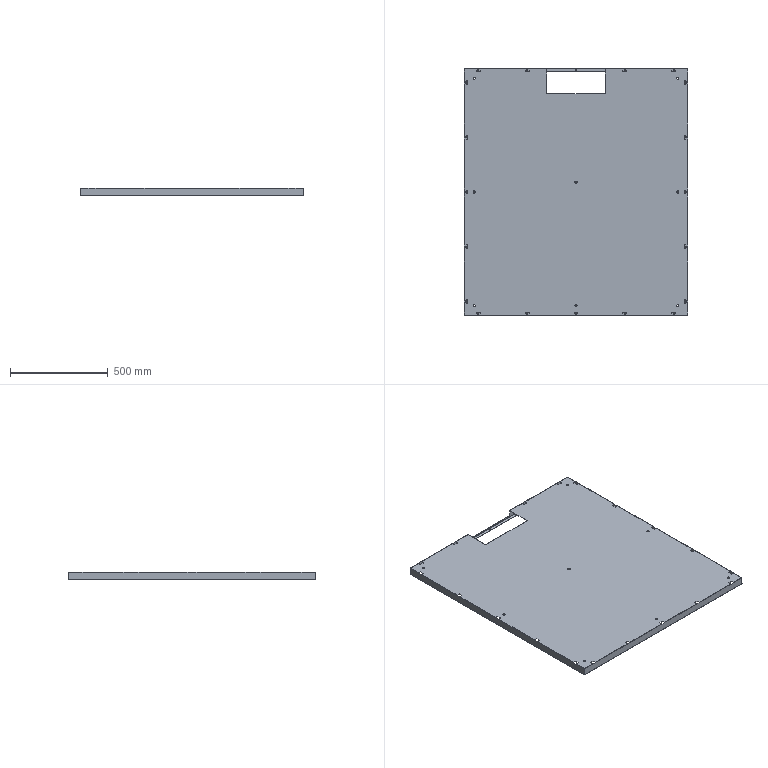Part | SolidWorks | features ICE 5, EdgeFlange 2, Cut 1, FlatPattern 1, SMBaseFlange 1, SheetMetal 1 | 1 solid | 376 faces | box 1139 x 1259 x 40 mm | volume 1637806 mm3 | plane 238 | cylinder 122 | spline 16 | commonest cylinder face diameters 7 x50 0.4 x28 2.4 x28 11 x16